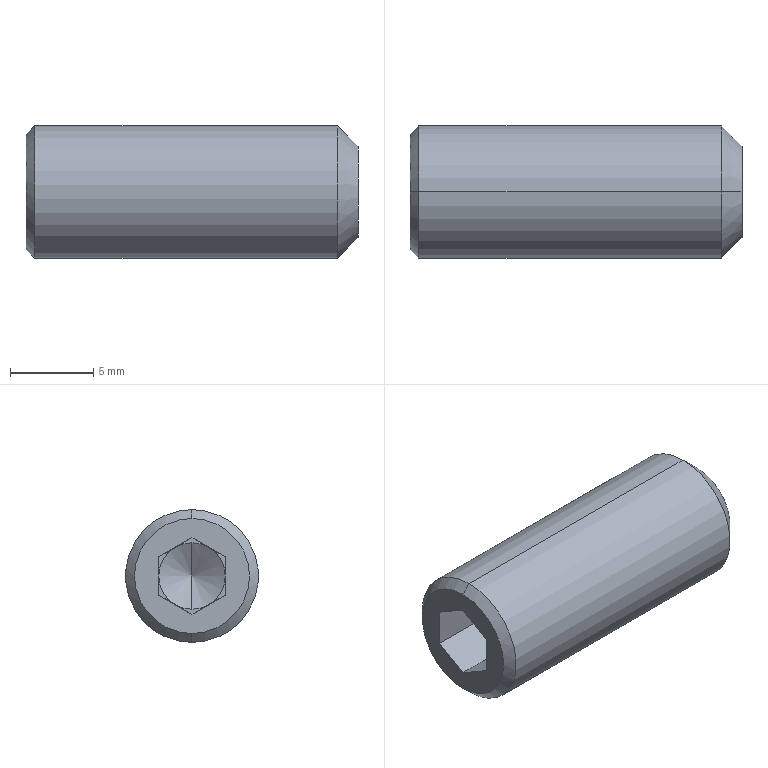Part | SolidWorks | features RevCut 2, Cut 1, LPattern 1, Revolution 1 | 1 solid | 22 faces | box 20 x 8 x 8 mm | volume 910.152 mm3 | plane 14 | cone 6 | cylinder 2 | commonest cylinder face diameters 8 x2
STEP:
#1=CARTESIAN_POINT('',(6.155,0.,0.));
#2=VERTEX_POINT('',#1);
#3=CARTESIAN_POINT('',(5.,0.,2.));
#4=VERTEX_POINT('',#3);
#5=CARTESIAN_POINT('',(6.155,0.,0.));
#6=DIRECTION('',(-0.5,0.,0.866));
#7=VECTOR('',#6,1000.);
#8=LINE('',#5,#7);
#9=EDGE_CURVE('',#2,#4,#8,.T.);
#10=ORIENTED_EDGE('',*,*,#9,.F.);
#11=CARTESIAN_POINT('',(5.,0.,-2.));
#12=VERTEX_POINT('',#11);
#13=CARTESIAN_POINT('',(6.155,0.,0.));
#14=DIRECTION('',(-0.5,0.,-0.866));
#15=VECTOR('',#14,1000.);
#16=LINE('',#13,#15);
#17=EDGE_CURVE('',#2,#12,#16,.T.);
#18=ORIENTED_EDGE('',*,*,#17,.T.);
#19=CARTESIAN_POINT('',(5.,-1.,-1.732));
#20=VERTEX_POINT('',#19);
#21=CARTESIAN_POINT('',(5.,0.,0.));
#22=DIRECTION('',(-1.,0.,0.));
#23=DIRECTION('',(0.,0.,1.));
#24=AXIS2_PLACEMENT_3D('',#21,#22,#23);
#25=CIRCLE('',#24,2.);
#26=EDGE_CURVE('',#12,#20,#25,.T.);
#27=ORIENTED_EDGE('',*,*,#26,.T.);
#28=CARTESIAN_POINT('',(5.,-2.,0.));
#29=VERTEX_POINT('',#28);
#30=CARTESIAN_POINT('',(5.,0.,0.));
#31=DIRECTION('',(-1.,0.,0.));
#32=DIRECTION('',(0.,0.,1.));
#33=AXIS2_PLACEMENT_3D('',#30,#31,#32);
#34=CIRCLE('',#33,2.);
#35=EDGE_CURVE('',#20,#29,#34,.T.);
#36=ORIENTED_EDGE('',*,*,#35,.T.);
#37=CARTESIAN_POINT('',(5.,-1.,1.732));
#38=VERTEX_POINT('',#37);
#39=CARTESIAN_POINT('',(5.,0.,0.));
#40=DIRECTION('',(-1.,0.,0.));
#41=DIRECTION('',(0.,0.,1.));
#42=AXIS2_PLACEMENT_3D('',#39,#40,#41);
#43=CIRCLE('',#42,2.);
#44=EDGE_CURVE('',#29,#38,#43,.T.);
#45=ORIENTED_EDGE('',*,*,#44,.T.);
#46=CARTESIAN_POINT('',(5.,0.,0.));
#47=DIRECTION('',(-1.,0.,0.));
#48=DIRECTION('',(0.,0.,1.));
#49=AXIS2_PLACEMENT_3D('',#46,#47,#48);
#50=CIRCLE('',#49,2.);
#51=EDGE_CURVE('',#38,#4,#50,.T.);
#52=ORIENTED_EDGE('',*,*,#51,.T.);
#53=EDGE_LOOP('',(#10,#18,#27,#36,#45,#52));
#54=FACE_OUTER_BOUND('',#53,.T.);
#55=CARTESIAN_POINT('',(-993.845,0.,0.));
#56=DIRECTION('',(-1.,0.,0.));
#57=DIRECTION('',(0.,0.,1.));
#58=AXIS2_PLACEMENT_3D('',#55,#56,#57);
#59=CONICAL_SURFACE('',#58,1732.051,1.047);
#60=ADVANCED_FACE('',(#54),#59,.F.);
#61=CARTESIAN_POINT('',(20.,0.,2.75));
#62=VERTEX_POINT('',#61);
#63=CARTESIAN_POINT('',(20.,0.,-2.75));
#64=VERTEX_POINT('',#63);
#65=CARTESIAN_POINT('',(20.,0.,0.));
#66=DIRECTION('',(-1.,0.,0.));
#67=DIRECTION('',(0.,0.,1.));
#68=AXIS2_PLACEMENT_3D('',#65,#66,#67);
#69=CIRCLE('',#68,2.75);
#70=EDGE_CURVE('',#62,#64,#69,.T.);
#71=ORIENTED_EDGE('',*,*,#70,.T.);
#72=CARTESIAN_POINT('',(18.75,0.,-4.));
#73=VERTEX_POINT('',#72);
#74=CARTESIAN_POINT('',(20.,0.,-2.75));
#75=DIRECTION('',(-0.7071,0.,-0.7071));
#76=VECTOR('',#75,1000.);
#77=LINE('',#74,#76);
#78=EDGE_CURVE('',#64,#73,#77,.T.);
#79=ORIENTED_EDGE('',*,*,#78,.T.);
#80=CARTESIAN_POINT('',(18.75,0.,4.));
#81=VERTEX_POINT('',#80);
#82=CARTESIAN_POINT('',(18.75,0.,0.));
#83=DIRECTION('',(-1.,0.,0.));
#84=DIRECTION('',(0.,0.,1.));
#85=AXIS2_PLACEMENT_3D('',#82,#83,#84);
#86=CIRCLE('',#85,4.);
#87=EDGE_CURVE('',#81,#73,#86,.T.);
#88=ORIENTED_EDGE('',*,*,#87,.F.);
#89=CARTESIAN_POINT('',(20.,0.,2.75));
#90=DIRECTION('',(-0.7071,0.,0.7071));
#91=VECTOR('',#90,1000.);
#92=LINE('',#89,#91);
#93=EDGE_CURVE('',#62,#81,#92,.T.);
#94=ORIENTED_EDGE('',*,*,#93,.F.);
#95=EDGE_LOOP('',(#71,#79,#88,#94));
#96=FACE_OUTER_BOUND('',#95,.T.);
#97=CARTESIAN_POINT('',(20.,0.,0.));
#98=DIRECTION('',(-1.,0.,0.));
#99=DIRECTION('',(0.,0.,1.));
#100=AXIS2_PLACEMENT_3D('',#97,#98,#99);
#101=CONICAL_SURFACE('',#100,2.75,0.7854);
#102=ADVANCED_FACE('',(#96),#101,.T.);
#103=ORIENTED_EDGE('',*,*,#87,.T.);
#104=CARTESIAN_POINT('',(0.536,0.,-4.));
#105=VERTEX_POINT('',#104);
#106=CARTESIAN_POINT('',(-0.2778,0.,-4.));
#107=DIRECTION('',(-1.,0.,0.));
#108=VECTOR('',#107,1000.);
#109=LINE('',#106,#108);
#110=EDGE_CURVE('',#73,#105,#109,.T.);
#111=ORIENTED_EDGE('',*,*,#110,.T.);
#112=CARTESIAN_POINT('',(0.536,0.,4.));
#113=VERTEX_POINT('',#112);
#114=CARTESIAN_POINT('',(0.536,0.,0.));
#115=DIRECTION('',(-1.,0.,0.));
#116=DIRECTION('',(0.,0.,1.));
#117=AXIS2_PLACEMENT_3D('',#114,#115,#116);
#118=CIRCLE('',#117,4.);
#119=EDGE_CURVE('',#113,#105,#118,.T.);
#120=ORIENTED_EDGE('',*,*,#119,.F.);
#121=CARTESIAN_POINT('',(-0.2778,0.,4.));
#122=DIRECTION('',(-1.,0.,0.));
#123=VECTOR('',#122,1000.);
#124=LINE('',#121,#123);
#125=EDGE_CURVE('',#81,#113,#124,.T.);
#126=ORIENTED_EDGE('',*,*,#125,.F.);
#127=EDGE_LOOP('',(#103,#111,#120,#126));
#128=FACE_OUTER_BOUND('',#127,.T.);
#129=CARTESIAN_POINT('',(-0.2778,0.,0.));
#130=DIRECTION('',(-1.,0.,0.));
#131=DIRECTION('',(0.,0.,1.));
#132=AXIS2_PLACEMENT_3D('',#129,#130,#131);
#133=CYLINDRICAL_SURFACE('',#132,4.);
#134=ADVANCED_FACE('',(#128),#133,.T.);
#135=CARTESIAN_POINT('',(0.,0.,3.464));
#136=VERTEX_POINT('',#135);
#137=CARTESIAN_POINT('',(0.,0.,-3.464));
#138=VERTEX_POINT('',#137);
#139=CARTESIAN_POINT('',(0.,0.,0.));
#140=DIRECTION('',(-1.,0.,0.));
#141=DIRECTION('',(0.,0.,1.));
#142=AXIS2_PLACEMENT_3D('',#139,#140,#141);
#143=CIRCLE('',#142,3.464);
#144=EDGE_CURVE('',#136,#138,#143,.T.);
#145=ORIENTED_EDGE('',*,*,#144,.F.);
#146=CARTESIAN_POINT('',(0.536,0.,4.));
#147=DIRECTION('',(0.7071,0.,0.7071));
#148=VECTOR('',#147,1000.);
#149=LINE('',#146,#148);
#150=EDGE_CURVE('',#136,#113,#149,.T.);
#151=ORIENTED_EDGE('',*,*,#150,.T.);
#152=ORIENTED_EDGE('',*,*,#119,.T.);
#153=CARTESIAN_POINT('',(0.536,0.,-4.));
#154=DIRECTION('',(0.7071,0.,-0.7071));
#155=VECTOR('',#154,1000.);
#156=LINE('',#153,#155);
#157=EDGE_CURVE('',#138,#105,#156,.T.);
#158=ORIENTED_EDGE('',*,*,#157,.F.);
#159=EDGE_LOOP('',(#145,#151,#152,#158));
#160=FACE_OUTER_BOUND('',#159,.T.);
#161=CARTESIAN_POINT('',(0.536,0.,0.));
#162=DIRECTION('',(1.,0.,0.));
#163=DIRECTION('',(0.,0.,-1.));
#164=AXIS2_PLACEMENT_3D('',#161,#162,#163);
#165=CONICAL_SURFACE('',#164,4.,0.7854);
#166=ADVANCED_FACE('',(#160),#165,.T.);
#167=CARTESIAN_POINT('',(5.,1.,1.732));
#168=VERTEX_POINT('',#167);
#169=CARTESIAN_POINT('',(5.,2.,0.));
#170=VERTEX_POINT('',#169);
#171=CARTESIAN_POINT('',(5.,0.,0.));
#172=DIRECTION('',(-1.,0.,0.));
#173=DIRECTION('',(0.,0.,1.));
#174=AXIS2_PLACEMENT_3D('',#171,#172,#173);
#175=CIRCLE('',#174,2.);
#176=EDGE_CURVE('',#168,#170,#175,.T.);
#177=ORIENTED_EDGE('',*,*,#176,.F.);
#178=CARTESIAN_POINT('',(5.,2.,1.155));
#179=VERTEX_POINT('',#178);
#180=CARTESIAN_POINT('',(5.,0.,2.309));
#181=DIRECTION('',(0.,0.866,-0.5));
#182=VECTOR('',#181,1000.);
#183=LINE('',#180,#182);
#184=EDGE_CURVE('',#168,#179,#183,.T.);
#185=ORIENTED_EDGE('',*,*,#184,.T.);
#186=CARTESIAN_POINT('',(5.,2.,1.155));
#187=DIRECTION('',(0.,0.,-1.));
#188=VECTOR('',#187,1000.);
#189=LINE('',#186,#188);
#190=EDGE_CURVE('',#179,#170,#189,.T.);
#191=ORIENTED_EDGE('',*,*,#190,.T.);
#192=EDGE_LOOP('',(#177,#185,#191));
#193=FACE_OUTER_BOUND('',#192,.T.);
#194=CARTESIAN_POINT('',(5.,0.,-2.309));
#195=DIRECTION('',(1.,0.,0.));
#196=DIRECTION('',(0.,0.,-1.));
#197=AXIS2_PLACEMENT_3D('',#194,#195,#196);
#198=PLANE('',#197);
#199=ADVANCED_FACE('',(#193),#198,.F.);
#200=CARTESIAN_POINT('',(5.,1.,-1.732));
#201=VERTEX_POINT('',#200);
#202=CARTESIAN_POINT('',(5.,0.,0.));
#203=DIRECTION('',(-1.,0.,0.));
#204=DIRECTION('',(0.,0.,1.));
#205=AXIS2_PLACEMENT_3D('',#202,#203,#204);
#206=CIRCLE('',#205,2.);
#207=EDGE_CURVE('',#170,#201,#206,.T.);
#208=ORIENTED_EDGE('',*,*,#207,.F.);
#209=CARTESIAN_POINT('',(5.,2.,-1.155));
#210=VERTEX_POINT('',#209);
#211=CARTESIAN_POINT('',(5.,2.,1.155));
#212=DIRECTION('',(0.,0.,-1.));
#213=VECTOR('',#212,1000.);
#214=LINE('',#211,#213);
#215=EDGE_CURVE('',#170,#210,#214,.T.);
#216=ORIENTED_EDGE('',*,*,#215,.T.);
#217=CARTESIAN_POINT('',(5.,2.,-1.155));
#218=DIRECTION('',(0.,-0.866,-0.5));
#219=VECTOR('',#218,1000.);
#220=LINE('',#217,#219);
#221=EDGE_CURVE('',#210,#201,#220,.T.);
#222=ORIENTED_EDGE('',*,*,#221,.T.);
#223=EDGE_LOOP('',(#208,#216,#222));
#224=FACE_OUTER_BOUND('',#223,.T.);
#225=CARTESIAN_POINT('',(5.,0.,-2.309));
#226=DIRECTION('',(1.,0.,0.));
#227=DIRECTION('',(0.,0.,-1.));
#228=AXIS2_PLACEMENT_3D('',#225,#226,#227);
#229=PLANE('',#228);
#230=ADVANCED_FACE('',(#224),#229,.F.);
#231=CARTESIAN_POINT('',(5.,0.,0.));
#232=DIRECTION('',(-1.,0.,0.));
#233=DIRECTION('',(0.,0.,1.));
#234=AXIS2_PLACEMENT_3D('',#231,#232,#233);
#235=CIRCLE('',#234,2.);
#236=EDGE_CURVE('',#201,#12,#235,.T.);
#237=ORIENTED_EDGE('',*,*,#236,.F.);
#238=CARTESIAN_POINT('',(5.,0.,-2.309));
#239=VERTEX_POINT('',#238);
#240=CARTESIAN_POINT('',(5.,2.,-1.155));
#241=DIRECTION('',(0.,-0.866,-0.5));
#242=VECTOR('',#241,1000.);
#243=LINE('',#240,#242);
#244=EDGE_CURVE('',#201,#239,#243,.T.);
#245=ORIENTED_EDGE('',*,*,#244,.T.);
#246=CARTESIAN_POINT('',(5.,0.,-2.309));
#247=DIRECTION('',(0.,-0.866,0.5));
#248=VECTOR('',#247,1000.);
#249=LINE('',#246,#248);
#250=EDGE_CURVE('',#239,#20,#249,.T.);
#251=ORIENTED_EDGE('',*,*,#250,.T.);
#252=ORIENTED_EDGE('',*,*,#26,.F.);
#253=EDGE_LOOP('',(#237,#245,#251,#252));
#254=FACE_OUTER_BOUND('',#253,.T.);
#255=CARTESIAN_POINT('',(5.,0.,-2.309));
#256=DIRECTION('',(1.,0.,0.));
#257=DIRECTION('',(0.,0.,-1.));
#258=AXIS2_PLACEMENT_3D('',#255,#256,#257);
#259=PLANE('',#258);
#260=ADVANCED_FACE('',(#254),#259,.F.);
#261=ORIENTED_EDGE('',*,*,#35,.F.);
#262=CARTESIAN_POINT('',(5.,-2.,-1.155));
#263=VERTEX_POINT('',#262);
#264=CARTESIAN_POINT('',(5.,0.,-2.309));
#265=DIRECTION('',(0.,-0.866,0.5));
#266=VECTOR('',#265,1000.);
#267=LINE('',#264,#266);
#268=EDGE_CURVE('',#20,#263,#267,.T.);
#269=ORIENTED_EDGE('',*,*,#268,.T.);
#270=CARTESIAN_POINT('',(5.,-2.,-1.155));
#271=DIRECTION('',(0.,0.,1.));
#272=VECTOR('',#271,1000.);
#273=LINE('',#270,#272);
#274=EDGE_CURVE('',#263,#29,#273,.T.);
#275=ORIENTED_EDGE('',*,*,#274,.T.);
#276=EDGE_LOOP('',(#261,#269,#275));
#277=FACE_OUTER_BOUND('',#276,.T.);
#278=CARTESIAN_POINT('',(5.,0.,-2.309));
#279=DIRECTION('',(1.,0.,0.));
#280=DIRECTION('',(0.,0.,-1.));
#281=AXIS2_PLACEMENT_3D('',#278,#279,#280);
#282=PLANE('',#281);
#283=ADVANCED_FACE('',(#277),#282,.F.);
#284=ORIENTED_EDGE('',*,*,#44,.F.);
#285=CARTESIAN_POINT('',(5.,-2.,1.155));
#286=VERTEX_POINT('',#285);
#287=CARTESIAN_POINT('',(5.,-2.,-1.155));
#288=DIRECTION('',(0.,0.,1.));
#289=VECTOR('',#288,1000.);
#290=LINE('',#287,#289);
#291=EDGE_CURVE('',#29,#286,#290,.T.);
#292=ORIENTED_EDGE('',*,*,#291,.T.);
#293=CARTESIAN_POINT('',(5.,-2.,1.155));
#294=DIRECTION('',(0.,0.866,0.5));
#295=VECTOR('',#294,1000.);
#296=LINE('',#293,#295);
#297=EDGE_CURVE('',#286,#38,#296,.T.);
#298=ORIENTED_EDGE('',*,*,#297,.T.);
#299=EDGE_LOOP('',(#284,#292,#298));
#300=FACE_OUTER_BOUND('',#299,.T.);
#301=CARTESIAN_POINT('',(5.,0.,-2.309));
#302=DIRECTION('',(1.,0.,0.));
#303=DIRECTION('',(0.,0.,-1.));
#304=AXIS2_PLACEMENT_3D('',#301,#302,#303);
#305=PLANE('',#304);
#306=ADVANCED_FACE('',(#300),#305,.F.);
#307=ORIENTED_EDGE('',*,*,#51,.F.);
#308=CARTESIAN_POINT('',(5.,0.,2.309));
#309=VERTEX_POINT('',#308);
#310=CARTESIAN_POINT('',(5.,-2.,1.155));
#311=DIRECTION('',(0.,0.866,0.5));
#312=VECTOR('',#311,1000.);
#313=LINE('',#310,#312);
#314=EDGE_CURVE('',#38,#309,#313,.T.);
#315=ORIENTED_EDGE('',*,*,#314,.T.);
#316=CARTESIAN_POINT('',(5.,0.,2.309));
#317=DIRECTION('',(0.,0.866,-0.5));
#318=VECTOR('',#317,1000.);
#319=LINE('',#316,#318);
#320=EDGE_CURVE('',#309,#168,#319,.T.);
#321=ORIENTED_EDGE('',*,*,#320,.T.);
#322=CARTESIAN_POINT('',(5.,0.,0.));
#323=DIRECTION('',(-1.,0.,0.));
#324=DIRECTION('',(0.,0.,1.));
#325=AXIS2_PLACEMENT_3D('',#322,#323,#324);
#326=CIRCLE('',#325,2.);
#327=EDGE_CURVE('',#4,#168,#326,.T.);
#328=ORIENTED_EDGE('',*,*,#327,.F.);
#329=EDGE_LOOP('',(#307,#315,#321,#328));
#330=FACE_OUTER_BOUND('',#329,.T.);
#331=CARTESIAN_POINT('',(5.,0.,-2.309));
#332=DIRECTION('',(1.,0.,0.));
#333=DIRECTION('',(0.,0.,-1.));
#334=AXIS2_PLACEMENT_3D('',#331,#332,#333);
#335=PLANE('',#334);
#336=ADVANCED_FACE('',(#330),#335,.F.);
#337=CARTESIAN_POINT('',(0.,-2.,-1.155));
#338=VERTEX_POINT('',#337);
#339=CARTESIAN_POINT('',(0.,-2.,1.155));
#340=VERTEX_POINT('',#339);
#341=CARTESIAN_POINT('',(0.,-2.,-1.155));
#342=DIRECTION('',(0.,0.,1.));
#343=VECTOR('',#342,1000.);
#344=LINE('',#341,#343);
#345=EDGE_CURVE('',#338,#340,#344,.T.);
#346=ORIENTED_EDGE('',*,*,#345,.F.);
#347=CARTESIAN_POINT('',(0.,0.,-2.309));
#348=VERTEX_POINT('',#347);
#349=CARTESIAN_POINT('',(0.,0.,-2.309));
#350=DIRECTION('',(0.,-0.866,0.5));
#351=VECTOR('',#350,1000.);
#352=LINE('',#349,#351);
#353=EDGE_CURVE('',#348,#338,#352,.T.);
#354=ORIENTED_EDGE('',*,*,#353,.F.);
#355=CARTESIAN_POINT('',(0.,2.,-1.155));
#356=VERTEX_POINT('',#355);
#357=CARTESIAN_POINT('',(0.,2.,-1.155));
#358=DIRECTION('',(0.,-0.866,-0.5));
#359=VECTOR('',#358,1000.);
#360=LINE('',#357,#359);
#361=EDGE_CURVE('',#356,#348,#360,.T.);
#362=ORIENTED_EDGE('',*,*,#361,.F.);
#363=CARTESIAN_POINT('',(0.,2.,1.155));
#364=VERTEX_POINT('',#363);
#365=CARTESIAN_POINT('',(0.,2.,1.155));
#366=DIRECTION('',(0.,0.,-1.));
#367=VECTOR('',#366,1000.);
#368=LINE('',#365,#367);
#369=EDGE_CURVE('',#364,#356,#368,.T.);
#370=ORIENTED_EDGE('',*,*,#369,.F.);
#371=CARTESIAN_POINT('',(0.,0.,2.309));
#372=VERTEX_POINT('',#371);
#373=CARTESIAN_POINT('',(0.,0.,2.309));
#374=DIRECTION('',(0.,0.866,-0.5));
#375=VECTOR('',#374,1000.);
#376=LINE('',#373,#375);
#377=EDGE_CURVE('',#372,#364,#376,.T.);
#378=ORIENTED_EDGE('',*,*,#377,.F.);
#379=CARTESIAN_POINT('',(0.,-2.,1.155));
#380=DIRECTION('',(0.,0.866,0.5));
#381=VECTOR('',#380,1000.);
#382=LINE('',#379,#381);
#383=EDGE_CURVE('',#340,#372,#382,.T.);
#384=ORIENTED_EDGE('',*,*,#383,.F.);
#385=EDGE_LOOP('',(#346,#354,#362,#370,#378,#384));
#386=FACE_BOUND('',#385,.T.);
#387=CARTESIAN_POINT('',(0.,0.,0.));
#388=DIRECTION('',(-1.,0.,0.));
#389=DIRECTION('',(0.,0.,1.));
#390=AXIS2_PLACEMENT_3D('',#387,#388,#389);
#391=CIRCLE('',#390,3.464);
#392=EDGE_CURVE('',#138,#136,#391,.T.);
#393=ORIENTED_EDGE('',*,*,#392,.T.);
#394=ORIENTED_EDGE('',*,*,#144,.T.);
#395=EDGE_LOOP('',(#393,#394));
#396=FACE_OUTER_BOUND('',#395,.T.);
#397=CARTESIAN_POINT('',(0.,3.464,0.));
#398=DIRECTION('',(1.,0.,0.));
#399=DIRECTION('',(0.,0.,-1.));
#400=AXIS2_PLACEMENT_3D('',#397,#398,#399);
#401=PLANE('',#400);
#402=ADVANCED_FACE('',(#386,#396),#401,.F.);
#403=ORIENTED_EDGE('',*,*,#150,.F.);
#404=ORIENTED_EDGE('',*,*,#392,.F.);
#405=ORIENTED_EDGE('',*,*,#157,.T.);
#406=CARTESIAN_POINT('',(0.536,0.,0.));
#407=DIRECTION('',(-1.,0.,0.));
#408=DIRECTION('',(0.,0.,1.));
#409=AXIS2_PLACEMENT_3D('',#406,#407,#408);
#410=CIRCLE('',#409,4.);
#411=EDGE_CURVE('',#105,#113,#410,.T.);
#412=ORIENTED_EDGE('',*,*,#411,.T.);
#413=EDGE_LOOP('',(#403,#404,#405,#412));
#414=FACE_OUTER_BOUND('',#413,.T.);
#415=CARTESIAN_POINT('',(0.536,0.,0.));
#416=DIRECTION('',(1.,0.,0.));
#417=DIRECTION('',(0.,0.,-1.));
#418=AXIS2_PLACEMENT_3D('',#415,#416,#417);
#419=CONICAL_SURFACE('',#418,4.,0.7854);
#420=ADVANCED_FACE('',(#414),#419,.T.);
#421=ORIENTED_EDGE('',*,*,#110,.F.);
#422=CARTESIAN_POINT('',(18.75,0.,0.));
#423=DIRECTION('',(-1.,0.,0.));
#424=DIRECTION('',(0.,0.,1.));
#425=AXIS2_PLACEMENT_3D('',#422,#423,#424);
#426=CIRCLE('',#425,4.);
#427=EDGE_CURVE('',#73,#81,#426,.T.);
#428=ORIENTED_EDGE('',*,*,#427,.T.);
#429=ORIENTED_EDGE('',*,*,#125,.T.);
#430=ORIENTED_EDGE('',*,*,#411,.F.);
#431=EDGE_LOOP('',(#421,#428,#429,#430));
#432=FACE_OUTER_BOUND('',#431,.T.);
#433=CARTESIAN_POINT('',(-0.2778,0.,0.));
#434=DIRECTION('',(-1.,0.,0.));
#435=DIRECTION('',(0.,0.,1.));
#436=AXIS2_PLACEMENT_3D('',#433,#434,#435);
#437=CYLINDRICAL_SURFACE('',#436,4.);
#438=ADVANCED_FACE('',(#432),#437,.T.);
#439=ORIENTED_EDGE('',*,*,#78,.F.);
#440=CARTESIAN_POINT('',(20.,0.,0.));
#441=DIRECTION('',(-1.,0.,0.));
#442=DIRECTION('',(0.,0.,1.));
#443=AXIS2_PLACEMENT_3D('',#440,#441,#442);
#444=CIRCLE('',#443,2.75);
#445=EDGE_CURVE('',#64,#62,#444,.T.);
#446=ORIENTED_EDGE('',*,*,#445,.T.);
#447=ORIENTED_EDGE('',*,*,#93,.T.);
#448=ORIENTED_EDGE('',*,*,#427,.F.);
#449=EDGE_LOOP('',(#439,#446,#447,#448));
#450=FACE_OUTER_BOUND('',#449,.T.);
#451=CARTESIAN_POINT('',(20.,0.,0.));
#452=DIRECTION('',(-1.,0.,0.));
#453=DIRECTION('',(0.,0.,1.));
#454=AXIS2_PLACEMENT_3D('',#451,#452,#453);
#455=CONICAL_SURFACE('',#454,2.75,0.7854);
#456=ADVANCED_FACE('',(#450),#455,.T.);
#457=ORIENTED_EDGE('',*,*,#70,.F.);
#458=ORIENTED_EDGE('',*,*,#445,.F.);
#459=EDGE_LOOP('',(#457,#458));
#460=FACE_OUTER_BOUND('',#459,.T.);
#461=CARTESIAN_POINT('',(20.,0.,0.));
#462=DIRECTION('',(-1.,0.,0.));
#463=DIRECTION('',(0.,0.,1.));
#464=AXIS2_PLACEMENT_3D('',#461,#462,#463);
#465=PLANE('',#464);
#466=ADVANCED_FACE('',(#460),#465,.F.);
#467=ORIENTED_EDGE('',*,*,#353,.T.);
#468=CARTESIAN_POINT('',(5.,-2.,-1.155));
#469=DIRECTION('',(-1.,0.,0.));
#470=VECTOR('',#469,1000.);
#471=LINE('',#468,#470);
#472=EDGE_CURVE('',#263,#338,#471,.T.);
#473=ORIENTED_EDGE('',*,*,#472,.F.);
#474=ORIENTED_EDGE('',*,*,#268,.F.);
#475=ORIENTED_EDGE('',*,*,#250,.F.);
#476=CARTESIAN_POINT('',(5.,0.,-2.309));
#477=DIRECTION('',(-1.,0.,0.));
#478=VECTOR('',#477,1000.);
#479=LINE('',#476,#478);
#480=EDGE_CURVE('',#239,#348,#479,.T.);
#481=ORIENTED_EDGE('',*,*,#480,.T.);
#482=EDGE_LOOP('',(#467,#473,#474,#475,#481));
#483=FACE_OUTER_BOUND('',#482,.T.);
#484=CARTESIAN_POINT('',(5.,0.,-2.309));
#485=DIRECTION('',(0.,-0.5,-0.866));
#486=DIRECTION('',(0.,0.866,-0.5));
#487=AXIS2_PLACEMENT_3D('',#484,#485,#486);
#488=PLANE('',#487);
#489=ADVANCED_FACE('',(#483),#488,.F.);
#490=ORIENTED_EDGE('',*,*,#361,.T.);
#491=ORIENTED_EDGE('',*,*,#480,.F.);
#492=ORIENTED_EDGE('',*,*,#244,.F.);
#493=ORIENTED_EDGE('',*,*,#221,.F.);
#494=CARTESIAN_POINT('',(5.,2.,-1.155));
#495=DIRECTION('',(-1.,0.,0.));
#496=VECTOR('',#495,1000.);
#497=LINE('',#494,#496);
#498=EDGE_CURVE('',#210,#356,#497,.T.);
#499=ORIENTED_EDGE('',*,*,#498,.T.);
#500=EDGE_LOOP('',(#490,#491,#492,#493,#499));
#501=FACE_OUTER_BOUND('',#500,.T.);
#502=CARTESIAN_POINT('',(5.,2.,-1.155));
#503=DIRECTION('',(0.,0.5,-0.866));
#504=DIRECTION('',(0.,0.866,0.5));
#505=AXIS2_PLACEMENT_3D('',#502,#503,#504);
#506=PLANE('',#505);
#507=ADVANCED_FACE('',(#501),#506,.F.);
#508=ORIENTED_EDGE('',*,*,#369,.T.);
#509=ORIENTED_EDGE('',*,*,#498,.F.);
#510=ORIENTED_EDGE('',*,*,#215,.F.);
#511=ORIENTED_EDGE('',*,*,#190,.F.);
#512=CARTESIAN_POINT('',(5.,2.,1.155));
#513=DIRECTION('',(-1.,0.,0.));
#514=VECTOR('',#513,1000.);
#515=LINE('',#512,#514);
#516=EDGE_CURVE('',#179,#364,#515,.T.);
#517=ORIENTED_EDGE('',*,*,#516,.T.);
#518=EDGE_LOOP('',(#508,#509,#510,#511,#517));
#519=FACE_OUTER_BOUND('',#518,.T.);
#520=CARTESIAN_POINT('',(5.,2.,1.155));
#521=DIRECTION('',(0.,1.,0.));
#522=DIRECTION('',(0.,0.,1.));
#523=AXIS2_PLACEMENT_3D('',#520,#521,#522);
#524=PLANE('',#523);
#525=ADVANCED_FACE('',(#519),#524,.F.);
#526=ORIENTED_EDGE('',*,*,#377,.T.);
#527=ORIENTED_EDGE('',*,*,#516,.F.);
#528=ORIENTED_EDGE('',*,*,#184,.F.);
#529=ORIENTED_EDGE('',*,*,#320,.F.);
#530=CARTESIAN_POINT('',(5.,0.,2.309));
#531=DIRECTION('',(-1.,0.,0.));
#532=VECTOR('',#531,1000.);
#533=LINE('',#530,#532);
#534=EDGE_CURVE('',#309,#372,#533,.T.);
#535=ORIENTED_EDGE('',*,*,#534,.T.);
#536=EDGE_LOOP('',(#526,#527,#528,#529,#535));
#537=FACE_OUTER_BOUND('',#536,.T.);
#538=CARTESIAN_POINT('',(5.,0.,2.309));
#539=DIRECTION('',(0.,0.5,0.866));
#540=DIRECTION('',(0.,-0.866,0.5));
#541=AXIS2_PLACEMENT_3D('',#538,#539,#540);
#542=PLANE('',#541);
#543=ADVANCED_FACE('',(#537),#542,.F.);
#544=ORIENTED_EDGE('',*,*,#383,.T.);
#545=ORIENTED_EDGE('',*,*,#534,.F.);
#546=ORIENTED_EDGE('',*,*,#314,.F.);
#547=ORIENTED_EDGE('',*,*,#297,.F.);
#548=CARTESIAN_POINT('',(5.,-2.,1.155));
#549=DIRECTION('',(-1.,0.,0.));
#550=VECTOR('',#549,1000.);
#551=LINE('',#548,#550);
#552=EDGE_CURVE('',#286,#340,#551,.T.);
#553=ORIENTED_EDGE('',*,*,#552,.T.);
#554=EDGE_LOOP('',(#544,#545,#546,#547,#553));
#555=FACE_OUTER_BOUND('',#554,.T.);
#556=CARTESIAN_POINT('',(5.,-2.,1.155));
#557=DIRECTION('',(0.,-0.5,0.866));
#558=DIRECTION('',(0.,-0.866,-0.5));
#559=AXIS2_PLACEMENT_3D('',#556,#557,#558);
#560=PLANE('',#559);
#561=ADVANCED_FACE('',(#555),#560,.F.);
#562=ORIENTED_EDGE('',*,*,#345,.T.);
#563=ORIENTED_EDGE('',*,*,#552,.F.);
#564=ORIENTED_EDGE('',*,*,#291,.F.);
#565=ORIENTED_EDGE('',*,*,#274,.F.);
#566=ORIENTED_EDGE('',*,*,#472,.T.);
#567=EDGE_LOOP('',(#562,#563,#564,#565,#566));
#568=FACE_OUTER_BOUND('',#567,.T.);
#569=CARTESIAN_POINT('',(5.,-2.,-1.155));
#570=DIRECTION('',(0.,-1.,0.));
#571=DIRECTION('',(0.,0.,-1.));
#572=AXIS2_PLACEMENT_3D('',#569,#570,#571);
#573=PLANE('',#572);
#574=ADVANCED_FACE('',(#568),#573,.F.);
#575=ORIENTED_EDGE('',*,*,#17,.F.);
#576=ORIENTED_EDGE('',*,*,#9,.T.);
#577=ORIENTED_EDGE('',*,*,#327,.T.);
#578=ORIENTED_EDGE('',*,*,#176,.T.);
#579=ORIENTED_EDGE('',*,*,#207,.T.);
#580=ORIENTED_EDGE('',*,*,#236,.T.);
#581=EDGE_LOOP('',(#575,#576,#577,#578,#579,#580));
#582=FACE_OUTER_BOUND('',#581,.T.);
#583=CARTESIAN_POINT('',(-993.845,0.,0.));
#584=DIRECTION('',(-1.,0.,0.));
#585=DIRECTION('',(0.,0.,1.));
#586=AXIS2_PLACEMENT_3D('',#583,#584,#585);
#587=CONICAL_SURFACE('',#586,1732.051,1.047);
#588=ADVANCED_FACE('',(#582),#587,.F.);
#589=CLOSED_SHELL('',(#60,#102,#134,#166,#199,#230,#260,#283,#306,#336,#402,#420,#438,#456,#466,#489,#507,#525,#543,#561,#574,#588));
#590=MANIFOLD_SOLID_BREP('',#589);
#591=CARTESIAN_POINT('',(0.,0.,0.));
#592=DIRECTION('',(0.,0.,1.));
#593=DIRECTION('',(1.,0.,0.));
#594=AXIS2_PLACEMENT_3D('',#591,#592,#593);
#595=(LENGTH_UNIT()NAMED_UNIT(*)SI_UNIT(.MILLI.,.METRE.));
#596=UNCERTAINTY_MEASURE_WITH_UNIT(LENGTH_MEASURE(0.00001),#595,'','');
#597=(NAMED_UNIT(*)PLANE_ANGLE_UNIT()SI_UNIT($,.RADIAN.));
#598=(NAMED_UNIT(*)SI_UNIT($,.STERADIAN.)SOLID_ANGLE_UNIT());
#599=(GEOMETRIC_REPRESENTATION_CONTEXT(3)GLOBAL_UNCERTAINTY_ASSIGNED_CONTEXT((#596))GLOBAL_UNIT_ASSIGNED_CONTEXT((#595,#597,#598))REPRESENTATION_CONTEXT('',''));
#600=ADVANCED_BREP_SHAPE_REPRESENTATION('',(#590,#594),#599);